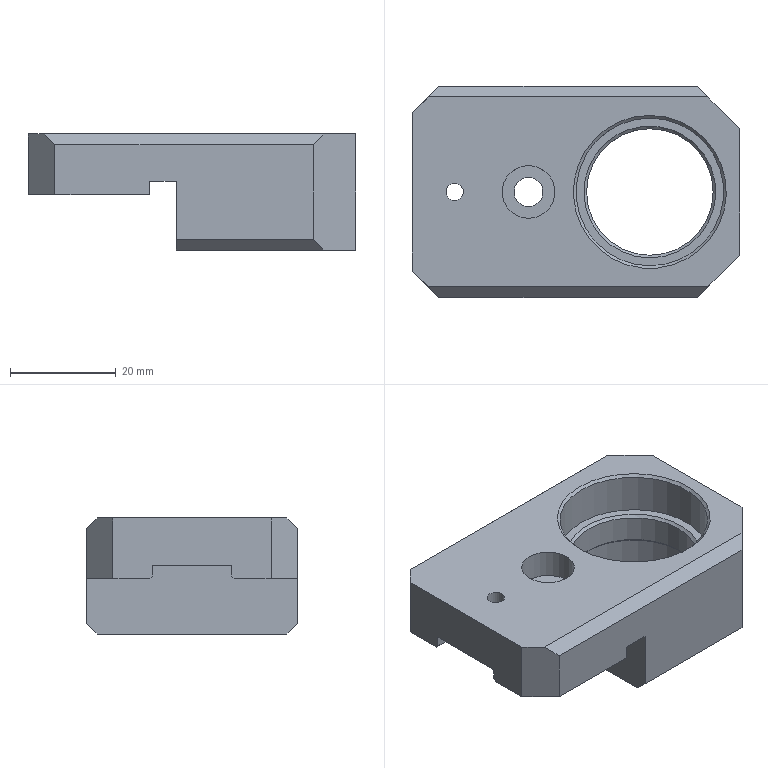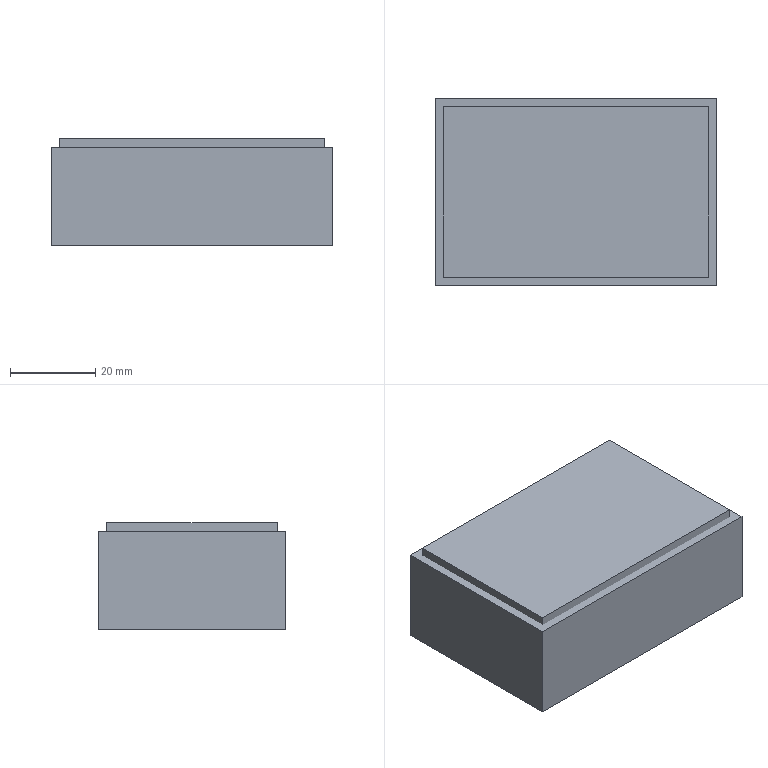CAM job | NX | 3-axis milling, drilling | part box 62 x 40 x 22 mm | stock box 66 x 44 x 25 mm
Tools:
number,name,description,diameter,corner_radius,flute_length,length,flutes
1,D63,Milling Tool-5 Parameters,63.0,0.0,50.0,75.0,2
6,D8A45,Milling Tool-5 Parameters,8.0,0.0,50.0,75.0,2
12,3.3ZT,Drilling Tool,3.3,0.0,35.0,50.0,2
22,5.5ZT,Drilling Tool,5.5,0.0,35.0,50.0,2
4,D10,Milling Tool-5 Parameters,10.0,0.0,50.0,75.0,2
2,D6,Milling Tool-5 Parameters,6.0,0.0,50.0,75.0,2
24,D4,Milling Tool-5 Parameters,4.0,0.0,50.0,75.0,2
Operations:
program,operation,operation_type,tool,method,geometry_group,spindle_rpm,surface_speed,feed_per_tooth,feed_cut,feed_plunge,cut_length_mm,path_length_mm,cut_time_min,machine_time_min
1,FLOOR_WALL,VolumeBased25DMillingOperation,D63,METHOD,A,6500.0,1286.0,0.1154,1500.0,100.0,141.0,195.0,0.094,0.0994
1,DRILLING,Operation,D8A45,METHOD,A,3500.0,65.0,0.0357,250.0,0.0,12.0,150.316,0.048,0.0618
1,DRILLING_COPY,Operation,3.3ZT,METHOD,A,1500.0,15.0,0.05,150.0,0.0,14.491,88.983,0.0966,0.1041
1,DRILLING_1,Operation,5.5ZT,METHOD,A,2000.0,26.0,0.05,200.0,0.0,15.152,90.305,0.0758,0.0833
1,ZLEVEL_PROFILE,ZLevelMilling,D10,METHOD,A,7000.0,219.0,0.2143,3000.0,1000.0,4964.605,5043.605,1.687,1.695
1,HOLE_MILLING,CylinderMilling,D10,METHOD,A,7000.0,0.0,0.0,2000.0,100.0,839.033,915.033,0.4195,0.4271
1,HOLE_MILLING_COPY,CylinderMilling,D10,METHOD,A,7000.0,0.0,0.0,2000.0,100.0,1040.997,1144.997,0.5205,0.5309
1,ZLEVEL_PROFILE_COPY,ZLevelMilling,D10,METHOD,A,7000.0,219.0,0.0714,1000.0,1000.0,551.986,790.565,0.552,0.5758
1,HOLE_MILLING_1,CylinderMilling,D6,METHOD,A,7000.0,131.0,0.1,1400.0,100.0,167.25,232.15,0.1195,0.126
1,PLANAR_MILL,PlanarMilling,D8A45,METHOD,A,7000.0,1495.0,0.0893,1250.0,100.0,338.007,635.014,0.2704,0.3001
1,PLANAR_MILL_COPY,PlanarMilling,D8A45,METHOD,A,7000.0,1495.0,0.0893,1250.0,100.0,403.683,874.52,0.3229,0.37
1,CUTTERCOMP4,CylinderMilling,D10,METHOD,A,7000.0,0.0,0.0714,1000.0,100.0,238.315,305.815,0.2383,0.2451
2,FLOOR_WALL_COPY,VolumeBased25DMillingOperation,D63,METHOD,B,6500.0,1286.0,0.1154,1500.0,100.0,411.0,829.001,0.274,0.3158
2,HOLE_MILLING_COPY_1,CylinderMilling,D10,METHOD,B,7000.0,0.0,0.0,2000.0,100.0,555.771,623.271,0.2779,0.2846
2,FLOOR_WALL_1,VolumeBased25DMillingOperation,D10,METHOD,B,7000.0,219.0,0.2143,3000.0,1000.0,3712.957,3903.325,1.264,1.283
2,FLOOR_WALL_1_COPY,VolumeBased25DMillingOperation,D10,METHOD,B,7000.0,219.0,0.0857,1200.0,1000.0,332.281,468.516,0.2781,0.2917
2,FLOOR_WALL_1_COPY_1,VolumeBased25DMillingOperation,D4,METHOD,B,7000.0,87.0,0.1429,2000.0,1000.0,1496.14,1605.789,0.7578,0.7687
2,FLOOR_WALL_1_COPY_COPY,VolumeBased25DMillingOperation,D4,METHOD,B,7000.0,219.0,0.0857,1200.0,1000.0,378.041,481.441,0.3171,0.3274
2,PLANAR_MILL_COPY_1,PlanarMilling,D8A45,METHOD,B,7000.0,1495.0,0.0893,1250.0,100.0,242.005,368.112,0.1936,0.2062
2,PLANAR_MILL_COPY_1_COPY,PlanarMilling,D8A45,METHOD,B,7000.0,1495.0,0.0893,1250.0,100.0,135.841,340.841,0.1087,0.1292
2,PLANAR_MILL_COPY_COPY,PlanarMilling,D8A45,METHOD,B,7000.0,1495.0,0.0893,1250.0,100.0,303.683,738.731,0.2429,0.2865
2,CUTTERCOMP4_COPY,CylinderMilling,D10,METHOD,B,7000.0,0.0,0.0714,1000.0,100.0,238.315,305.815,0.2383,0.2451